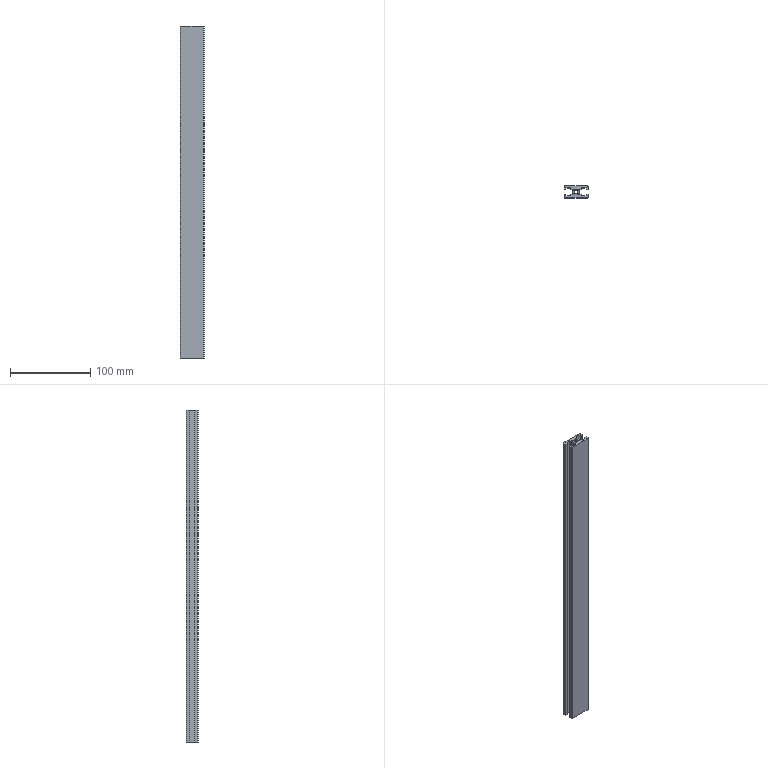Part | NX | features BREP 1 | 1 solid | 53 faces | box 30 x 15 x 415 mm | volume 100085 mm3 | plane 38 | cylinder 15 | commonest cylinder face diameters 1 x6 5 x5 2 x4